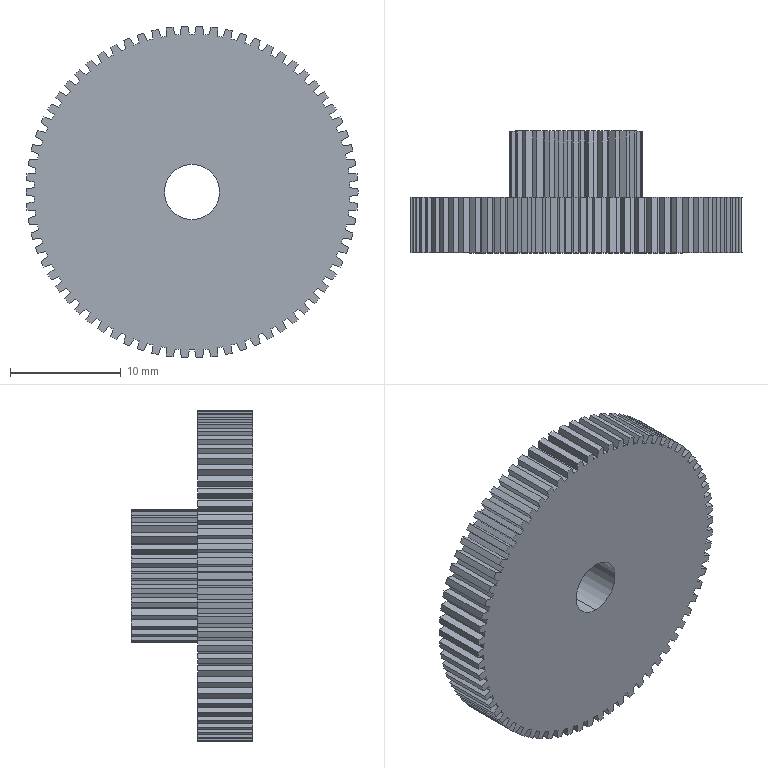Part | SolidWorks | features BaseBody 1 | 1 solid | 399 faces | box 30 x 11 x 29.991 mm | volume 3758 mm3 | cylinder 200 | plane 199 | commonest cylinder face diameters 28.552 x71 30 x70 12 x29 10.5 x28 5 x2